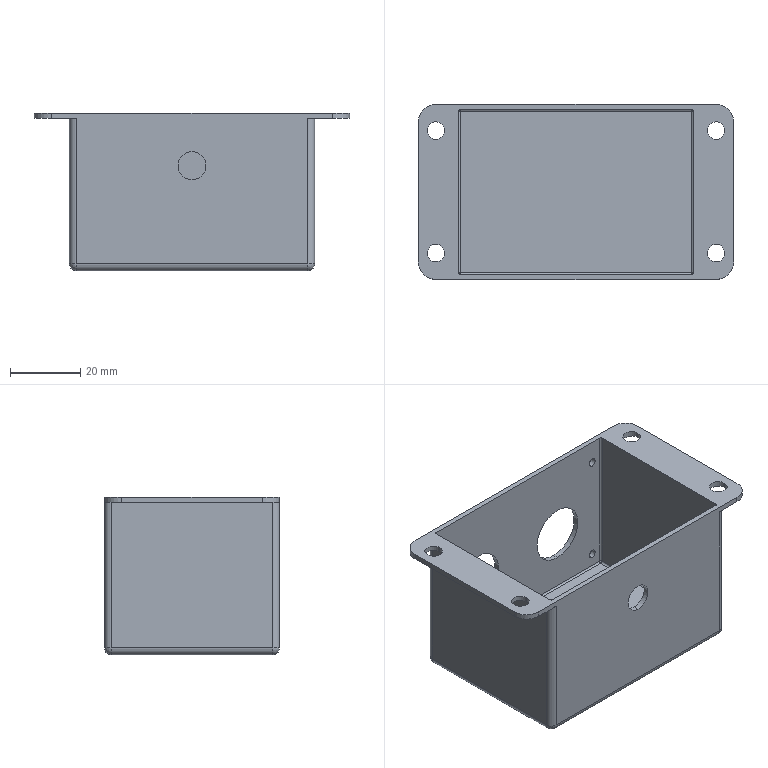Part | SolidWorks | features ICE 4, Fillet 2, Emboss 1, Extrusion 1, HoleWzd 1, Shell 1 | 1 solid | 65 faces | box 90 x 50 x 45 mm | volume 20794 mm3 | cylinder 42 | plane 15 | sphere 8 | commonest cylinder face diameters 1 x8 2.5 x8 4 x8 5 x8 10 x4 16.5 x4